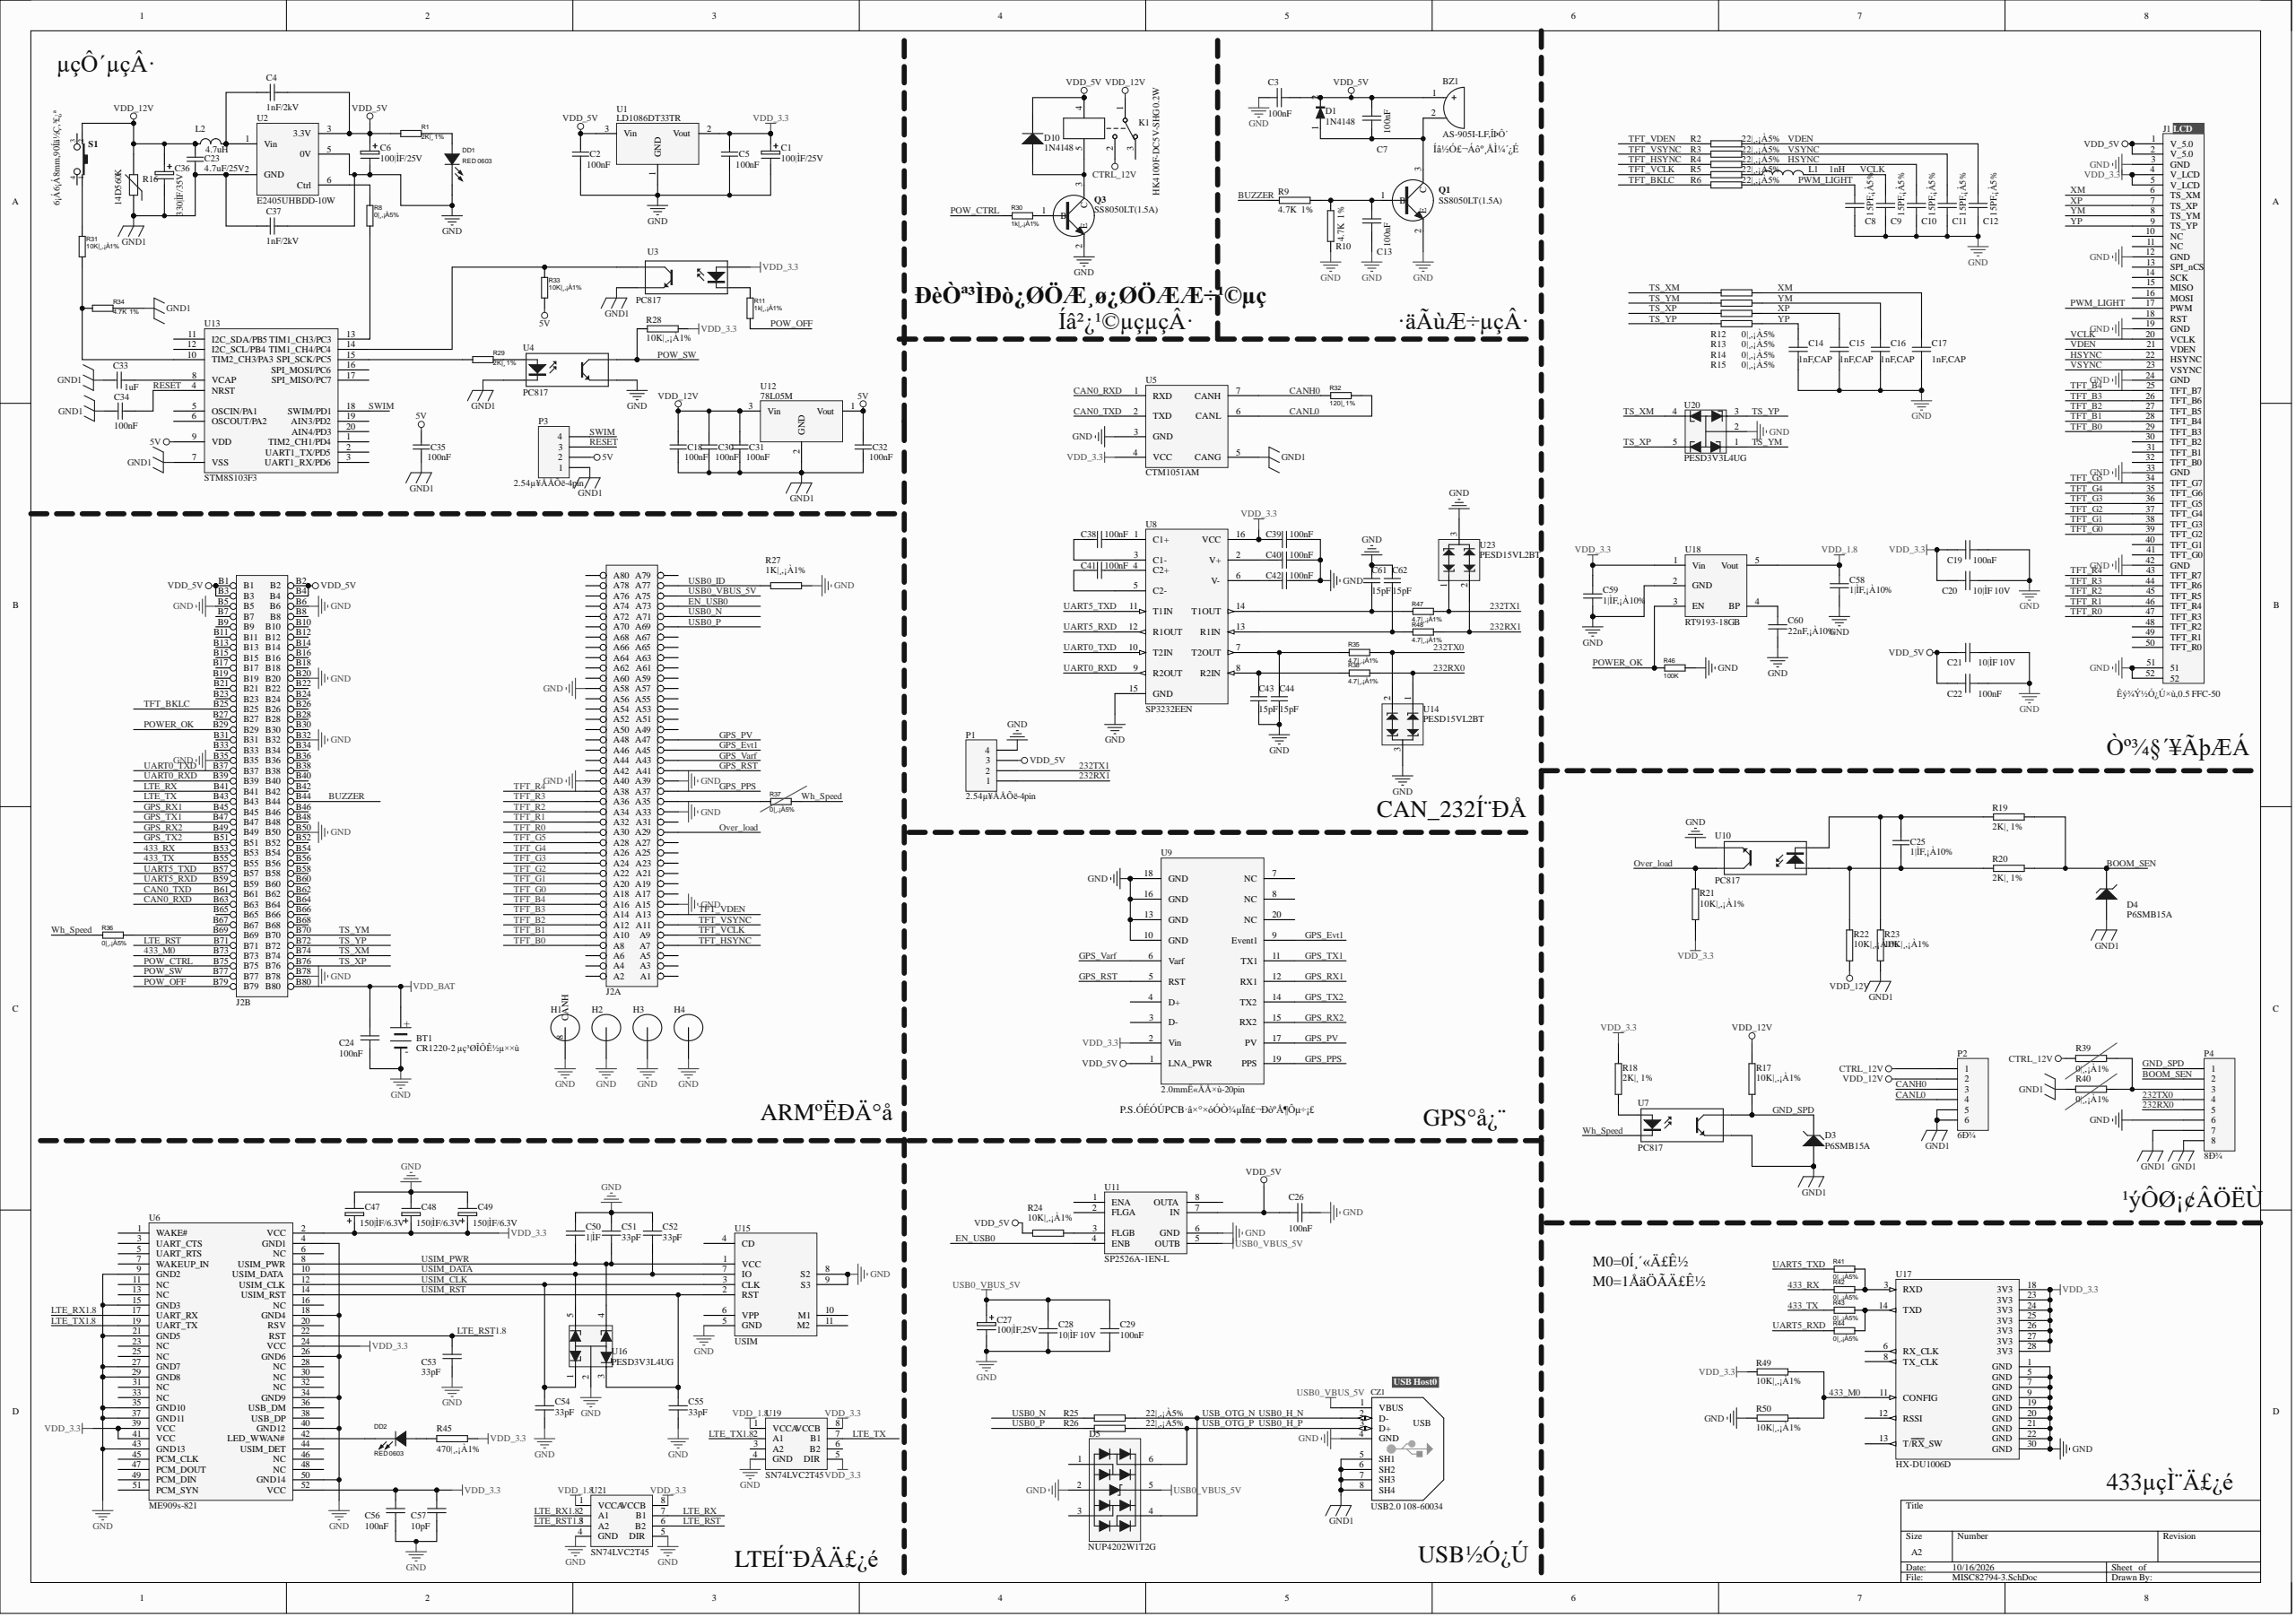Circuit board | Altium Designer | 157 parts | 133 nets
Bill of materials:
Comment,Description,Designator,Footprint,LibRef,Quantity
"BATTERY","2P,间距1.25mm,Wafer凹槽边框,90°,FPC2-49T","BT1","BATTERY-1220-1","1.10.05.0096","1"
"BUZZER2","AS-905I-LF,无源,Ф9×4.8mm,常州立翔,RoHS","BZ1","XH2.5-2P","1.06.09.0016","1"
"100|ÌF/25V","220|ÌF,16V,§¶6.3¡Á7mm,,珠海华冠,RoHS","C1, C6","RB6.3*7","1.02.11.0018","2"
"100nF","Capacitor (Semiconductor SIM Model), 0.1|ÌF,¡À10%,X5R,25V,0402,RoHS, Capacitor","C2, C3, C5, C7, C13, C18, C19, C22, C24, C26, C29, C30, C31, C32, C34, C35, C38, C39, C40, C41, C42, C56","0805C","Cap Semi, 1.02.17.0020, Cap","22"
"1nF/2kV","Capacitor (Semiconductor SIM Model)","C4, C37","C1206","Cap Semi","2"
"15PF,¡À5%","15PF,¡À5%,50V,COG,0402,RoHS","C8, C9, C10, C11, C12","0805C","1.02.17.0005","5"
"1nF,CAP","1nF,CAP,CER,1000PF,50V,CDG,GRM1555C1H102JA01D,0402,MURATA,RoHS","C14, C15, C16, C17","0805C","1.02.17.0021","4"
"10|ÌF 10V","10uF,6.3V,X5R,GRM188R60J106ME47D,0603,Murata,RoHS, 106,10|ÌF,¡À10%,10V,X5R,0805,RoHS","C20, C21, C28","0805C","1.02.01.0065, 1.02.02.0055","3"
"4.7uF/25V","Capacitor (Semiconductor SIM Model)","C23","C1206","Cap Semi","1"
"1|ÌF,¡À10%","Capacitor, 1uF,¡À10%,X7R,25V","C25, C58, C59","0805C","Cap, 1.02.17.0020","3"
"100|ÌF,25V","220|ÌF,16V,§¶6.3¡Á7mm,,珠海华冠,RoHS","C27","CAPPRD250W45D630H800P","1.02.11.0018","1"
"1uF","Capacitor (Semiconductor SIM Model)","C33","0805C","Cap Semi","1"
"330|ÌF/35V","220|ÌF,16V,§¶6.3¡Á7mm,,珠海华冠,RoHS","C36","CAPPR5.0-10X16-0.8","1.02.11.0018","1"
"15pF","Capacitor","C43, C44, C61, C62","0805C","Cap","4"
"150|ÌF/6.3V","220|ÌF,16V,§¶6.3¡Á7mm,,珠海华冠,RoHS","C47, C48, C49","CT3528-B","1.02.11.0018","3"
"1|ÌF","0.1|ÌF,¡À10%,X5R,25V,0402,RoHS","C50","0805C","1.02.17.0020","1"
"33pF","0.1|ÌF,¡À10%,X5R,25V,0402,RoHS","C51, C52, C53, C54, C55","0805C","1.02.17.0020","5"
"10pF","0.1|ÌF,¡À10%,X5R,25V,0402,RoHS","C57","0805C","1.02.17.0020","1"
"22nF,¡À10%","22nF,¡À10%,X5R,50V","C60","0805C","1.02.17.0020","1"
"USB","3190004-H73-R,USB-A插座,立式,90°,THT,WCON,RoHS","CZ1","USB-1400","1.10.12.0012","1"
"1N4148","1N4148,SOD-323,RoHS, Default Diode","D1, D10","SMD-D4148","1.04.07.0027, Diode","2"
"P6SMB15A","Zener Diode","D3, D4","DO-214","D Zener","2"
"NUP4202W1","NUP4202W1T2G,SC-88,ON,RoHS","D5","SOT-363","1.05.10.0376","1"
"RED 0603","","DD1, DD2","LED0805","LED_0","2"
"Hole","Hole","H1, H2, H3, H4","HOLE-3.2","Hole","4"
"FPC-50","数据接口座,0.5FFC-50,SMD,下接,RoHS","J1","FFC0.5-50P-A","1.10.01.0028","1"
"HEADER 40X2","DF12D(3.0)-80DP-0.5V(81),Fmale,SMT,HRS,RoHS","J2","AM3352B","","1"
"HK4100F-DC5V-SHG 0.2W","Single-Pole Dual-Throw Relay","K1","HK4100F","Relay-SPDT","1"
"1nH","BM02Y190S40R,0402,丰晶,RoHS","L1","0805R","1.03.03.0022","1"
"4.7uH","Inductor","L2","SLF6045","Inductor","1"
"2.54单排针-4pin","Header, 4-Pin","P1, P3","HDR1X4","Header 4","2"
"6芯","Header, 6-Pin","P2","BBD-06PMFP-LC7001","Header 6","1"
"8芯","Header, 8-Pin","P4","BDU-08PMFP-LC7001","Header 8","1"
"SS8050LT(1.5A)","SS8050LT(1.5A),SOT-23,江苏长电,RoHS","Q1, Q3","SOT-23","1.04.09.0001","2"
"2K|¸ 1%","","R1, R18, R19, R20, R29","0805R","RES, 1.01.17.0004","5"
"22|¸,¡À5%","22|¸,¡À5%,0402,RALEC,RoHS","R2, R3, R4, R5, R6, R25, R26","0805R","1.01.17.0023","7"
"0|¸,¡À5%","[NoValue], 0|¸,¡À5%,0402,RALEC,RoHS","R8, R12, R13, R14, R15, R36, R37, R41, R42, R43, R44","0805R","RES, 1.01.17.0004","11"
"4.7K  1%","","R9, R10, R34","0805R","1.01.17.0019, RES","3"
"1k|¸,¡À1%","[NoValue], 10K,¡À5%,0402,RALEC,RoHS","R11, R27, R30","0805R","RES, 1.01.17.0006","3"
"14D560K","Varistor (Voltage-Sensitive Resistor)","R16","14D560K","Res Varistor","1"
"10K|¸,¡À1%","[NoValue], 10K,¡À5%,0402,RALEC,RoHS","R17, R21, R22, R23, R24, R28, R31, R33, R49, R50","0805R","1.01.17.0004, 1.01.17.0006, RES","10"
"120|¸ 1%","","R32","0805R","RES","1"
"4.7|¸,¡À1%","","R35, R38, R47, R48","0805R","RES","4"
"0|¸,¡À1%","10K,¡À5%,0402,RALEC,RoHS","R39, R40","0805R","1.01.17.0006","2"
"470|¸,¡À1%","10K,¡À5%,0402,RALEC,RoHS","R45","0805R","1.01.17.0006","1"
"100K","","R46","0805R","RES","1"
"SW-PB4P","6×6×5.0mm,黑色,SMD,,*","S1","SWICH4.5","","1"
"LD1086DT33TR","","U1","DPAK","VOLTREG1","1"
"E2405UHBDD-10W","","U2","E2403UHBDD","E2403UHBDD-10W","1"
"PC817","Optoisolator","U3, U4, U7, U10","SMD-4","TLP281-1","4"
"CTM1051AM","CTM1051AM","U5","CTM1051AM","CTM1051AM","1"
"ME909s-821","ME909s-821","U6","","ME909s-821","1"
"SP3232EEN","","U8","SOP16-6.6","SP202ECT","1"
"2.0mm双排座-20pin","OEMStar","U9","20PIN-OEM_STARA","OEMStar","1"
"SP2526A","","U11","SOIC127P600X175-8N","1.05.09.0064","1"
"78L05M","","U12","SOT-89","VOLTREG1","1"
"STM8S103F3","","U13","TSOP65P640X120-20N","STM8S103F3","1"
"PESD15VL2BT","","U14, U23","SOT-23","PESD12VL2BT","2"
"USIM","USIM","U15","","USIM","1"
"PESD3V3L4UG","PESD3V3L4UG,SOT-353,NXP,RoHS","U16, U20","SOT-353","1.05.10.0265","2"
"HX-DU1006D","HX-DU1006D","U17","HX-DU1006D","HX-DU1006D","1"
"RT9193-18GB","RT9193","U18","SOT23-5","RT9193","1"
"SN74LVC2T45","SN74LVC2T45","U19, U21","","SN74LVC2T45","2"
Netlist (Protel format):
[
BT1
BATTERY-1220-1
BATTERY



]
[
BZ1
XH2.5-2P
BUZZER2



]
[
C1
RB6.3*7
100|ÌF/25V



]
[
C2
0805C
100nF



]
[
C3
0805C
100nF



]
[
C4
C1206
1nF/2kV



]
[
C5
0805C
100nF



]
[
C6
RB6.3*7
100|ÌF/25V



]
[
C7
0805C
100nF



]
[
C8
0805C
15PF,¡À5%



]
[
C9
0805C
15PF,¡À5%



]
[
C10
0805C
15PF,¡À5%



]
[
C11
0805C
15PF,¡À5%



]
[
C12
0805C
15PF,¡À5%



]
[
C13
0805C
100nF



]
[
C14
0805C
1nF,CAP



]
[
C15
0805C
1nF,CAP



]
[
C16
0805C
1nF,CAP



]
[
C17
0805C
1nF,CAP



]
[
C18
0805C
100nF



]
[
C19
0805C
100nF



]
[
C20
0805C
10|ÌF 10V



]
[
C21
0805C
10|ÌF 10V



]
[
C22
0805C
100nF



]
[
C23
C1206
4.7uF/25V



]
[
C24
0805C
100nF



]
[
C25
0805C
1|ÌF,¡À10%



]
[
C26
0805C
100nF



]
[
C27
CAPPRD250W45D630H800P
100|ÌF,25V



]
[
C28
0805C
10|ÌF 10V



]
[
C29
0805C
100nF



]
[
C30
0805C
100nF



]
[
C31
0805C
100nF



]
[
C32
0805C
100nF



]
[
C33
0805C
1uF



]
[
C34
0805C
100nF



]
[
C35
0805C
100nF



]
[
C36
CAPPR5.0-10X16-0.8
330|ÌF/35V



]
[
C37
C1206
1nF/2kV



]
[
C38
0805C
100nF



]
[
C39
0805C
100nF



]
[
C40
0805C
100nF



]
[
C41
0805C
100nF



]
[
C42
0805C
100nF



]
[
C43
0805C
15pF



]
[
C44
0805C
15pF



]
[
C47
CT3528-B
150|ÌF/6.3V



]
[
C48
CT3528-B
150|ÌF/6.3V



]
[
C49
CT3528-B
150|ÌF/6.3V



]
[
C50
0805C
1|ÌF



]
[
C51
0805C
33pF



]
[
C52
0805C
33pF



]
[
C53
0805C
33pF



]
[
C54
0805C
33pF



]
[
C55
0805C
33pF



]
[
C56
0805C
100nF



]
[
C57
0805C
10pF



]
[
C58
0805C
1|ÌF,¡À10%



]
[
C59
0805C
1|ÌF,¡À10%



]
[
C60
0805C
22nF,¡À10%



]
[
C61
0805C
15pF



]
[
C62
0805C
15pF



]
[
CZ1
USB-1400
USB



]
[
D1
SMD-D4148
1N4148



]
[
D3
DO-214
P6SMB15A



]
[
D4
DO-214
P6SMB15A



]
[
D5
SOT-363
NUP4202W1



]
[
D10
SMD-D4148
1N4148



]
[
DD1
LED0805
RED 0603



]
[
DD2
LED0805
RED 0603



]
[
H1
HOLE-3.2
Hole



]
[
H2
HOLE-3.2
Hole



]
[
H3
HOLE-3.2
Hole



]
[
H4
HOLE-3.2
Hole



]
[
J1
FFC0.5-50P-A
FPC-50



]
[
J2
AM3352B
HEADER 40X2



]
[
K1
HK4100F
HK4100F-DC5V-SHG 0.2W



]
[
L1
0805R
1nH



]
[
L2
SLF6045
4.7uH



]
[
P1
HDR1X4
2.54单排针-4pin



]
[
P2
BBD-06PMFP-LC7001
6芯



]
[
P3
HDR1X4
2.54单排针-4pin



]
[
P4
BDU-08PMFP-LC7001
8芯



]
[
Q1
SOT-23
SS8050LT(1.5A)



]
[
Q3
SOT-23
SS8050LT(1.5A)



]
[
R1
0805R
2K|¸ 1%



]
[
R2
0805R
22|¸,¡À5%



]
[
R3
0805R
22|¸,¡À5%



]
[
R4
0805R
22|¸,¡À5%



]
[
R5
0805R
22|¸,¡À5%



]
[
R6
0805R
22|¸,¡À5%



]
[
R8
0805R
0|¸,¡À5%



]
[
R9
0805R
4.7K  1%



]
[
R10
0805R
4.7K  1%



]
[
R11
0805R
1k|¸,¡À1%



]
[
R12
0805R
0|¸,¡À5%



]
[
R13
0805R
0|¸,¡À5%



]
[
R14
0805R
0|¸,¡À5%



]
[
R15
0805R
0|¸,¡À5%



]
[
R16
14D560K
14D560K



]
[
R17
0805R
10K|¸,¡À1%



]
[
R18
0805R
2K|¸ 1%



]
[
R19
0805R
2K|¸ 1%



]
[
R20
0805R
2K|¸ 1%



]
[
R21
0805R
10K|¸,¡À1%



]
[
R22
0805R
10K|¸,¡À1%



]
[
R23
0805R
10K|¸,¡À1%



]
[
R24
0805R
10K|¸,¡À1%



]
[
R25
0805R
22|¸,¡À5%



]
[
R26
0805R
22|¸,¡À5%



]
[
R27
0805R
1K|¸,¡À1%



]
[
R28
0805R
10K|¸,¡À1%



]
[
R29
0805R
2K|¸ 1%



]
[
R30
0805R
1k|¸,¡À1%



]
[
R31
0805R
10K|¸,¡À1%



]
[
R32
0805R
120|¸ 1%



]
[
R33
0805R
10K|¸,¡À1%



]
[
R34
0805R
4.7K  1%



]
[
R35
0805R
4.7|¸,¡À1%



]
[
R36
0805R
0|¸,¡À5%



]
[
R37
0805R
0|¸,¡À5%



]
[
R38
0805R
4.7|¸,¡À1%



]
[
R39
0805R
0|¸,¡À1%



]
[
R40
0805R
0|¸,¡À1%



]
[
R41
0805R
0|¸,¡À5%



]
[
R42
0805R
0|¸,¡À5%



]
[
R43
0805R
0|¸,¡À5%



]
[
R44
0805R
0|¸,¡À5%



]
[
R45
0805R
470|¸,¡À1%



]
[
R46
0805R
100K



]
[
R47
0805R
4.7|¸,¡À1%



]
[
R48
0805R
4.7|¸,¡À1%



]
[
R49
0805R
10K|¸,¡À1%



]
[
R50
0805R
10K|¸,¡À1%



]
[
S1
SWICH4.5
SW-PB4P



]
[
U1
DPAK
LD1086DT33TR



]
[
U2
E2403UHBDD
E2405UHBDD-10W



]
[
U3
SMD-4
PC817



]
[
U4
SMD-4
PC817



]
[
U5
CTM1051AM
CTM1051AM



]
[
U6

ME909s-821



]
[
U7
SMD-4
PC817



]
[
U8
SOP16-6.6
SP3232EEN



]
[
U9
20PIN-OEM_STARA
2.0mm双排座-20pin



]
[
U10
SMD-4
PC817



]
[
U11
SOIC127P600X175-8N
SP2526A



]
[
U12
SOT-89
78L05M



]
[
U13
TSOP65P640X120-20N
STM8S103F3



]
[
U14
SOT-23
PESD15VL2BT



]
[
U15

USIM



]
[
U16
SOT-353
PESD3V3L4UG



]
[
U17
HX-DU1006D
HX-DU1006D



]
[
U18
SOT23-5
RT9193-18GB



]
[
U19

SN74LVC2T45



]
[
U20
SOT-353
PESD3V3L4UG



]
[
U21

SN74LVC2T45



]
[
U23
SOT-23
PESD15VL2BT



]
(
YP
C14-1
J1-9
R15-2
)
(
YM
C16-1
J1-8
R13-2
)
(
XP
C15-1
J1-7
R14-2
)
(
XM
C17-1
J1-6
R12-2
)
(
Wh_Speed
R36-1
R37-1
U7-2
)
(
VSYNC
C11-1
J1-23
R3-2
)
(
VDEN
C12-1
J1-21
R2-2
)
(
VDD_BAT
BT1-1
C24-1
J2-B80
)
(
VDD_12V
C18-1
C23-2
C30-1
C31-1
C36-1
K1-1
L2-1
P2-2
R16-2
R17-2
R22-2
S1-2
U12-3
)
(
VDD_5V
BZ1-1
C2-1
C3-1
C4-2
C6-1
C7-2
C21-1
C22-2
C26-2
D1-2
D10-2
J1-1
J1-2
J2-B1
J2-B2
J2-B3
J2-B4
K1-4
P1-3
R1-2
R24-2
U1-3
U2-3
U9-1
U11-7
)
(
VDD_3.3
C1-1
C5-1
C19-2
C20-2
C39-1
C47-1
C48-1
C49-1
C56-1
C57-1
C59-2
J1-4
J1-5
R18-1
R21-1
R28-1
R45-1
R49-2
U1-2
U3-1
U5-4
U6-2
U6-24
U6-39
U6-41
U6-52
U8-16
U9-2
U17-18
U17-23
U17-24
U17-25
U17-26
U17-27
U17-28
U18-1
U19-5
U19-8
U21-8
)
(
VDD_1.8
C58-2
U18-5
U19-1
U21-1
)
(
VCLK
C9-1
J1-20
L1-2
)
(
USIM_RST
C55-2
U6-14
U15-2
U16-3
)
(
USIM_PWR
C50-1
C51-1
U6-8
U15-1
U16-4
)
(
USIM_DATA
C52-1
U6-10
U15-7
U16-5
)
(
USIM_CLK
C54-2
U6-12
U15-3
U16-1
)
(
USB0_VBUS_5V
C27-1
C28-1
C29-1
CZ1-1
D5-5
J2-A75
U11-5
)
(
USB0_P
J2-A69
R26-1
)
(
USB0_N
J2-A71
R25-1
)
(
USB0_ID
J2-A77
R27-2
)
(
USB0_H_P
CZ1-3
D5-6
R26-2
)
(
USB0_H_N
CZ1-2
D5-4
R25-2
)
(
UART5_TXD
J2-B57
R41-1
U8-11
)
(
UART5_RXD
J2-B59
R44-1
U8-12
)
(
UART0_TXD
J2-B37
U8-10
)
(
UART0_RXD
J2-B39
U8-9
)
(
TS_YP
J2-B72
R15-1
U20-3
)
(
TS_YM
J2-B70
R13-1
U20-1
)
(
TS_XP
J2-B76
R14-1
U20-5
)
(
TS_XM
J2-B74
R12-1
U20-4
)
(
TFT_VSYNC
J2-A11
R3-1
)
(
TFT_VDEN
J2-A13
R2-1
)
(
TFT_VCLK
J2-A9
R5-1
)
(
TFT_R4
J1-43
J2-A38
)
(
TFT_R3
J1-44
J2-A36
)
(
TFT_R2
J1-45
J2-A34
)
(
TFT_R1
J1-46
J2-A32
)
(
TFT_R0
J1-47
J2-A30
)
(
TFT_HSYNC
J2-A7
R4-1
)
(
TFT_G5
J1-34
J2-A28
)
(
TFT_G4
J1-35
J2-A26
)
(
TFT_G3
J1-36
J2-A24
)
(
TFT_G2
J1-37
J2-A22
)
(
TFT_G1
J1-38
J2-A20
)
(
TFT_G0
J1-39
J2-A18
)
(
TFT_BKLC
J2-B25
R6-1
)
(
TFT_B4
J1-25
J2-A16
)
(
TFT_B3
J1-26
J2-A14
)
(
TFT_B2
J1-27
J2-A12
)
(
TFT_B1
J1-28
J2-A10
)
(
TFT_B0
J1-29
J2-A8
)
(
SWIM
P3-4
U13-18
)
(
RESET
C34-2
P3-3
U13-4
)
(
PWM_LIGHT
C8-1
J1-17
R6-2
)
(
POWER_OK
J2-B29
R46-1
U18-3
)
(
POW_SW
J2-B77
R28-2
U4-4
)
(
POW_OFF
J2-B79
R11-1
)
(
POW_CTRL
J2-B75
R30-1
)
(
Over_load
J2-A29
R21-2
U10-4
)
(
NetR43_2
R43-2
R44-2
U17-14
)
(
NetR41_2
R41-2
R42-2
U17-3
)
(
NetR33_2
R33-2
U3-4
U13-14
)
(
NetR31_2
R31-2
R34-2
U13-10
)
(
NetR31_1
R31-1
S1-1
)
(
NetR29_2
R29-2
U13-15
)
(
NetR29_1
R29-1
U4-1
)
(
NetR24_1
R24-1
U11-3
)
(
NetR18_2
R18-2
U7-1
)
(
NetR11_2
R11-2
U3-2
)
(
NetR8_2
R8-2
U13-13
)
(
NetR8_1
R8-1
U2-6
)
(
NetQ3_1
Q3-1
R30-2
)
(
NetP4_3
P4-3
R39-1
R40-1
)
(
NetL1_1
L1-1
R5-2
)
(
NetJ2_B69
J2-B69
R36-2
)
(
NetJ2_A35
J2-A35
R37-2
)
(
NetDD2_2
DD2-2
U6-42
)
(
NetDD2_1
DD2-1
R45-2
)
(
NetDD1_1
DD1-1
R1-1
)
(
NetD10_1
D10-1
K1-5
Q3-3
)
(
NetC62_2
C62-2
R48-2
U8-13
)
(
NetC61_2
C61-2
R47-2
U8-14
)
(
NetC60_2
C60-2
U18-4
)
(
NetC44_1
C44-1
R35-2
U8-7
)
(
NetC43_1
C43-1
R38-2
U8-8
)
(
NetC42_1
C42-1
U8-6
)
(
NetC41_2
C41-2
U8-4
)
(
NetC41_1
C41-1
U8-5
)
(
NetC40_1
C40-1
U8-2
)
(
NetC38_2
C38-2
U8-1
)
(
NetC38_1
C38-1
U8-3
)
(
NetC33_2
C33-2
U13-8
)
(
NetC25_2
C25-2
R19-2
R23-1
U10-2
)
(
NetC25_1
C25-1
R20-2
R22-1
U10-1
)
(
NetC13_2
C13-2
Q1-1
R9-2
R10-2
)
(
NetC4_1
C4-1
L2-2
U2-1
)
(
NetBZ1_2
BZ1-2
C7-1
D1-1
Q1-3
)
(
LTE_TX1.8
U6-19
U19-2
)
(
LTE_TX
J2-B43
U19-7
)
(
LTE_RX1.8
U6-17
U21-2
)
(
LTE_RX
J2-B41
U21-7
)
(
LTE_RST1.8
C53-1
U6-22
U21-3
)
(
LTE_RST
J2-B71
U21-6
)
(
HSYNC
C10-1
J1-22
R4-2
)
(
GPS_Varf
J2-A43
U9-6
)
(
GPS_TX2
J2-B51
U9-14
)
(
GPS_TX1
J2-B47
U9-11
)
(
GPS_RX2
J2-B49
U9-15
)
(
GPS_RX1
J2-B45
U9-12
)
(
GPS_RST
J2-A41
U9-5
)
(
GPS_PV
J2-A47
U9-17
)
(
GPS_PPS
J2-A37
U9-19
)
(
GPS_Evt1
J2-A45
U9-9
)
(
GND_SPD
D3-2
P4-1
R17-1
U7-4
)
(
GND1
C18-2
C23-1
C30-2
C31-2
C32-2
C33-1
C34-1
C35-2
C36-2
C37-1
CZ1-5
CZ1-6
CZ1-7
CZ1-8
D3-1
D4-1
P2-5
P2-6
P3-1
P4-7
P4-8
R16-1
R23-2
R34-1
R40-2
U2-2
U3-3
U4-2
U5-5
U7-3
U12-2
U13-7
)
(
GND
BT1-2
C1-2
C2-2
C3-2
C5-2
C6-2
C8-2
C9-2
C10-2
C11-2
C12-2
C13-1
C14-2
C15-2
C16-2
C17-2
C19-1
C20-1
C21-2
C22-1
C24-2
C26-1
C27-2
C28-2
C29-2
C37-2
C39-2
C40-2
C42-2
C43-2
C44-2
C47-2
C48-2
C49-2
C50-2
C51-2
C52-2
C53-2
C54-1
C55-1
C56-2
C57-2
C58-1
C59-1
C60-1
C61-1
C62-1
CZ1-4
D5-2
DD1-2
H1-8
H2-8
H3-8
H4-8
J1-3
J1-12
J1-19
J1-24
J1-33
J1-42
J1-51
J1-52
J2-A15
J2-A33
J2-A39
J2-A40
J2-A58
J2-B5
J2-B6
J2-B20
J2-B32
J2-B35
J2-B50
J2-B78
P1-4
P4-6
Q1-2
Q3-2
R10-1
R27-1
R46-2
R50-2
U1-1
U2-5
U4-3
U5-3
U6-4
U6-9
U6-15
U6-18
U6-21
U6-26
U6-27
U6-29
U6-34
U6-35
U6-37
U6-40
U6-43
U6-50
U8-15
U9-10
U9-13
U9-16
U9-18
U10-3
U11-6
U14-3
U15-5
U15-8
U15-9
U16-2
U17-1
U17-5
U17-7
U17-9
U17-19
U17-20
U17-21
U17-22
U17-30
U18-2
U19-4
U20-2
U21-4
U21-5
U23-3
)
(
EN_USB0
J2-A73
U11-4
)
(
CTRL_12V
K1-2
P2-1
R39-2
)
(
CANL0
P2-4
R32-2
U5-6
)
(
CANH0
P2-3
R32-1
U5-7
)
(
CAN0_TXD
J2-B61
U5-2
)
(
CAN0_RXD
J2-B63
U5-1
)
(
BUZZER
J2-B44
R9-1
)
(
BOOM_SEN
D4-2
P4-2
R19-1
R20-1
)
(
433_TX
J2-B55
R43-1
)
(
433_RX
J2-B53
R42-1
)
(
433_M0
J2-B73
R49-1
R50-1
U17-11
)
(
232TX1
P1-2
R47-1
U23-1
)
(
232TX0
P4-4
R35-1
U14-2
)
(
232RX1
P1-1
R48-1
U23-2
)
(
232RX0
P4-5
R38-1
U14-1
)
(
5V
C32-1
C35-1
P3-2
R33-1
U12-1
U13-9
)